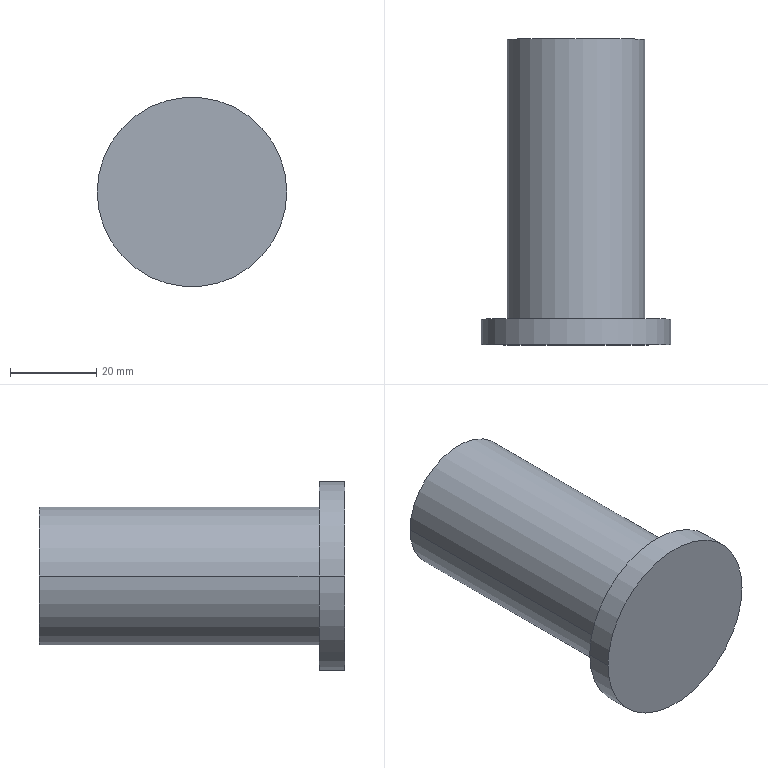Part | STEP file | Main ejector | 1 solid | 7 faces | box 44 x 71 x 44 mm | volume 61399 mm3 | cylinder 4 | plane 3 | commonest cylinder face diameters 32 x2 44 x2
STEP:
#1=CARTESIAN_POINT('',(0.,0.,0.));
#2=DIRECTION('',(0.,0.,1.));
#3=DIRECTION('',(1.,0.,0.));
#4=AXIS2_PLACEMENT_3D('',#1,#2,#3);
#5=CARTESIAN_POINT('',(-16.,6.,0.));
#6=VERTEX_POINT('',#5);
#7=CARTESIAN_POINT('',(16.,6.,0.));
#8=VERTEX_POINT('',#7);
#9=CARTESIAN_POINT('',(0.,6.,0.));
#10=DIRECTION('',(0.,1.,0.));
#11=DIRECTION('',(-1.,0.,0.));
#12=AXIS2_PLACEMENT_3D('',#9,#10,#11);
#13=CIRCLE('',#12,16.);
#14=CARTESIAN_POINT('',(0.,71.,0.));
#15=DIRECTION('',(0.,1.,0.));
#16=DIRECTION('',(-1.,0.,0.));
#17=AXIS2_PLACEMENT_3D('',#14,#15,#16);
#18=CYLINDRICAL_SURFACE('',#17,16.);
#19=CARTESIAN_POINT('',(0.,-65.));
#20=DIRECTION('',(1.,0.));
#21=VECTOR('',#20,1.);
#22=LINE('',#19,#21);
#23=(GEOMETRIC_REPRESENTATION_CONTEXT(2)PARAMETRIC_REPRESENTATION_CONTEXT()REPRESENTATION_CONTEXT('',''));
#24=DEFINITIONAL_REPRESENTATION('',(#22),#23);
#25=PCURVE('',#18,#24);
#26=CARTESIAN_POINT('',(-22.,6.,0.));
#27=DIRECTION('',(0.,1.,0.));
#28=DIRECTION('',(-1.,0.,0.));
#29=AXIS2_PLACEMENT_3D('',#26,#27,#28);
#30=PLANE('',#29);
#31=CARTESIAN_POINT('',(-22.,0.));
#32=DIRECTION('',(1.,0.));
#33=AXIS2_PLACEMENT_2D('',#31,#32);
#34=CIRCLE('',#33,16.);
#35=(GEOMETRIC_REPRESENTATION_CONTEXT(2)PARAMETRIC_REPRESENTATION_CONTEXT()REPRESENTATION_CONTEXT('',''));
#36=DEFINITIONAL_REPRESENTATION('',(#34),#35);
#37=PCURVE('',#30,#36);
#38=SURFACE_CURVE('',#13,(#25,#37),.PCURVE_S1.);
#39=EDGE_CURVE('',#6,#8,#38,.T.);
#40=ORIENTED_EDGE('',*,*,#39,.T.);
#41=CARTESIAN_POINT('',(16.,71.,0.));
#42=VERTEX_POINT('',#41);
#43=CARTESIAN_POINT('',(16.,71.,0.));
#44=DIRECTION('',(0.,1.,0.));
#45=VECTOR('',#44,1.);
#46=LINE('',#43,#45);
#47=CARTESIAN_POINT('',(3.142,0.));
#48=DIRECTION('',(0.,1.));
#49=VECTOR('',#48,1.);
#50=LINE('',#47,#49);
#51=(GEOMETRIC_REPRESENTATION_CONTEXT(2)PARAMETRIC_REPRESENTATION_CONTEXT()REPRESENTATION_CONTEXT('',''));
#52=DEFINITIONAL_REPRESENTATION('',(#50),#51);
#53=PCURVE('',#18,#52);
#54=CARTESIAN_POINT('',(0.,71.,0.));
#55=DIRECTION('',(0.,1.,0.));
#56=DIRECTION('',(-1.,0.,0.));
#57=AXIS2_PLACEMENT_3D('',#54,#55,#56);
#58=CYLINDRICAL_SURFACE('',#57,16.);
#59=CARTESIAN_POINT('',(3.142,0.));
#60=DIRECTION('',(0.,1.));
#61=VECTOR('',#60,1.);
#62=LINE('',#59,#61);
#63=(GEOMETRIC_REPRESENTATION_CONTEXT(2)PARAMETRIC_REPRESENTATION_CONTEXT()REPRESENTATION_CONTEXT('',''));
#64=DEFINITIONAL_REPRESENTATION('',(#62),#63);
#65=PCURVE('',#58,#64);
#66=SURFACE_CURVE('',#46,(#53,#65),.PCURVE_S1.);
#67=EDGE_CURVE('',#8,#42,#66,.T.);
#68=ORIENTED_EDGE('',*,*,#67,.T.);
#69=CARTESIAN_POINT('',(-16.,71.,0.));
#70=VERTEX_POINT('',#69);
#71=CARTESIAN_POINT('',(0.,71.,0.));
#72=DIRECTION('',(0.,1.,0.));
#73=DIRECTION('',(-1.,0.,0.));
#74=AXIS2_PLACEMENT_3D('',#71,#72,#73);
#75=CIRCLE('',#74,16.);
#76=CARTESIAN_POINT('',(0.,0.));
#77=DIRECTION('',(1.,0.));
#78=VECTOR('',#77,1.);
#79=LINE('',#76,#78);
#80=(GEOMETRIC_REPRESENTATION_CONTEXT(2)PARAMETRIC_REPRESENTATION_CONTEXT()REPRESENTATION_CONTEXT('',''));
#81=DEFINITIONAL_REPRESENTATION('',(#79),#80);
#82=PCURVE('',#18,#81);
#83=CARTESIAN_POINT('',(-16.,71.,0.));
#84=DIRECTION('',(0.,1.,0.));
#85=DIRECTION('',(-1.,0.,0.));
#86=AXIS2_PLACEMENT_3D('',#83,#84,#85);
#87=PLANE('',#86);
#88=CARTESIAN_POINT('',(-16.,0.));
#89=DIRECTION('',(1.,0.));
#90=AXIS2_PLACEMENT_2D('',#88,#89);
#91=CIRCLE('',#90,16.);
#92=(GEOMETRIC_REPRESENTATION_CONTEXT(2)PARAMETRIC_REPRESENTATION_CONTEXT()REPRESENTATION_CONTEXT('',''));
#93=DEFINITIONAL_REPRESENTATION('',(#91),#92);
#94=PCURVE('',#87,#93);
#95=SURFACE_CURVE('',#75,(#82,#94),.PCURVE_S1.);
#96=EDGE_CURVE('',#70,#42,#95,.T.);
#97=ORIENTED_EDGE('',*,*,#96,.F.);
#98=CARTESIAN_POINT('',(-16.,71.,0.));
#99=DIRECTION('',(0.,1.,0.));
#100=VECTOR('',#99,1.);
#101=LINE('',#98,#100);
#102=CARTESIAN_POINT('',(0.,0.));
#103=DIRECTION('',(0.,1.));
#104=VECTOR('',#103,1.);
#105=LINE('',#102,#104);
#106=(GEOMETRIC_REPRESENTATION_CONTEXT(2)PARAMETRIC_REPRESENTATION_CONTEXT()REPRESENTATION_CONTEXT('',''));
#107=DEFINITIONAL_REPRESENTATION('',(#105),#106);
#108=PCURVE('',#18,#107);
#109=CARTESIAN_POINT('',(6.283,0.));
#110=DIRECTION('',(0.,1.));
#111=VECTOR('',#110,1.);
#112=LINE('',#109,#111);
#113=(GEOMETRIC_REPRESENTATION_CONTEXT(2)PARAMETRIC_REPRESENTATION_CONTEXT()REPRESENTATION_CONTEXT('',''));
#114=DEFINITIONAL_REPRESENTATION('',(#112),#113);
#115=PCURVE('',#58,#114);
#116=SURFACE_CURVE('',#101,(#108,#115),.PCURVE_S1.);
#117=EDGE_CURVE('',#6,#70,#116,.T.);
#118=ORIENTED_EDGE('',*,*,#117,.F.);
#119=EDGE_LOOP('',(#40,#68,#97,#118));
#120=FACE_BOUND('',#119,.T.);
#121=ADVANCED_FACE('',(#120),#18,.T.);
#122=CARTESIAN_POINT('',(-22.,0.,0.));
#123=VERTEX_POINT('',#122);
#124=CARTESIAN_POINT('',(22.,0.,0.));
#125=VERTEX_POINT('',#124);
#126=CARTESIAN_POINT('',(0.,0.,0.));
#127=DIRECTION('',(0.,1.,0.));
#128=DIRECTION('',(-1.,0.,0.));
#129=AXIS2_PLACEMENT_3D('',#126,#127,#128);
#130=CIRCLE('',#129,22.);
#131=CARTESIAN_POINT('',(0.,71.,0.));
#132=DIRECTION('',(0.,1.,0.));
#133=DIRECTION('',(-1.,0.,0.));
#134=AXIS2_PLACEMENT_3D('',#131,#132,#133);
#135=CYLINDRICAL_SURFACE('',#134,22.);
#136=CARTESIAN_POINT('',(0.,-71.));
#137=DIRECTION('',(1.,0.));
#138=VECTOR('',#137,1.);
#139=LINE('',#136,#138);
#140=(GEOMETRIC_REPRESENTATION_CONTEXT(2)PARAMETRIC_REPRESENTATION_CONTEXT()REPRESENTATION_CONTEXT('',''));
#141=DEFINITIONAL_REPRESENTATION('',(#139),#140);
#142=PCURVE('',#135,#141);
#143=CARTESIAN_POINT('',(0.,0.,0.));
#144=DIRECTION('',(0.,-1.,0.));
#145=DIRECTION('',(1.,0.,0.));
#146=AXIS2_PLACEMENT_3D('',#143,#144,#145);
#147=PLANE('',#146);
#148=CARTESIAN_POINT('',(-22.,0.));
#149=CARTESIAN_POINT('',(-22.,38.105));
#150=CARTESIAN_POINT('',(11.,19.053));
#151=CARTESIAN_POINT('',(44.,0.));
#152=CARTESIAN_POINT('',(11.,-19.053));
#153=CARTESIAN_POINT('',(-22.,-38.105));
#154=CARTESIAN_POINT('',(-22.,0.));
#155=(BOUNDED_CURVE()B_SPLINE_CURVE(2,(#148,#149,#150,#151,#152,#153,#154),.UNSPECIFIED.,.T.,.F.)B_SPLINE_CURVE_WITH_KNOTS((1,2,2,2,2,1),(-2.094,0.,2.094,4.189,6.283,8.378),.UNSPECIFIED.)CURVE()GEOMETRIC_REPRESENTATION_ITEM()RATIONAL_B_SPLINE_CURVE((1.,0.5,1.,0.5,1.,0.5,1.))REPRESENTATION_ITEM(''));
#156=(GEOMETRIC_REPRESENTATION_CONTEXT(2)PARAMETRIC_REPRESENTATION_CONTEXT()REPRESENTATION_CONTEXT('',''));
#157=DEFINITIONAL_REPRESENTATION('',(#155),#156);
#158=PCURVE('',#147,#157);
#159=SURFACE_CURVE('',#130,(#142,#158),.PCURVE_S1.);
#160=EDGE_CURVE('',#123,#125,#159,.T.);
#161=ORIENTED_EDGE('',*,*,#160,.T.);
#162=CARTESIAN_POINT('',(22.,6.,0.));
#163=VERTEX_POINT('',#162);
#164=CARTESIAN_POINT('',(22.,71.,0.));
#165=DIRECTION('',(0.,1.,0.));
#166=VECTOR('',#165,1.);
#167=LINE('',#164,#166);
#168=CARTESIAN_POINT('',(3.142,0.));
#169=DIRECTION('',(0.,1.));
#170=VECTOR('',#169,1.);
#171=LINE('',#168,#170);
#172=(GEOMETRIC_REPRESENTATION_CONTEXT(2)PARAMETRIC_REPRESENTATION_CONTEXT()REPRESENTATION_CONTEXT('',''));
#173=DEFINITIONAL_REPRESENTATION('',(#171),#172);
#174=PCURVE('',#135,#173);
#175=CARTESIAN_POINT('',(0.,71.,0.));
#176=DIRECTION('',(0.,1.,0.));
#177=DIRECTION('',(-1.,0.,0.));
#178=AXIS2_PLACEMENT_3D('',#175,#176,#177);
#179=CYLINDRICAL_SURFACE('',#178,22.);
#180=CARTESIAN_POINT('',(3.142,0.));
#181=DIRECTION('',(0.,1.));
#182=VECTOR('',#181,1.);
#183=LINE('',#180,#182);
#184=(GEOMETRIC_REPRESENTATION_CONTEXT(2)PARAMETRIC_REPRESENTATION_CONTEXT()REPRESENTATION_CONTEXT('',''));
#185=DEFINITIONAL_REPRESENTATION('',(#183),#184);
#186=PCURVE('',#179,#185);
#187=SURFACE_CURVE('',#167,(#174,#186),.PCURVE_S1.);
#188=EDGE_CURVE('',#125,#163,#187,.T.);
#189=ORIENTED_EDGE('',*,*,#188,.T.);
#190=CARTESIAN_POINT('',(-22.,6.,0.));
#191=VERTEX_POINT('',#190);
#192=CARTESIAN_POINT('',(0.,6.,0.));
#193=DIRECTION('',(0.,1.,0.));
#194=DIRECTION('',(-1.,0.,0.));
#195=AXIS2_PLACEMENT_3D('',#192,#193,#194);
#196=CIRCLE('',#195,22.);
#197=CARTESIAN_POINT('',(0.,-65.));
#198=DIRECTION('',(1.,0.));
#199=VECTOR('',#198,1.);
#200=LINE('',#197,#199);
#201=(GEOMETRIC_REPRESENTATION_CONTEXT(2)PARAMETRIC_REPRESENTATION_CONTEXT()REPRESENTATION_CONTEXT('',''));
#202=DEFINITIONAL_REPRESENTATION('',(#200),#201);
#203=PCURVE('',#135,#202);
#204=CARTESIAN_POINT('',(-22.,0.));
#205=DIRECTION('',(1.,0.));
#206=AXIS2_PLACEMENT_2D('',#204,#205);
#207=CIRCLE('',#206,22.);
#208=(GEOMETRIC_REPRESENTATION_CONTEXT(2)PARAMETRIC_REPRESENTATION_CONTEXT()REPRESENTATION_CONTEXT('',''));
#209=DEFINITIONAL_REPRESENTATION('',(#207),#208);
#210=PCURVE('',#30,#209);
#211=SURFACE_CURVE('',#196,(#203,#210),.PCURVE_S1.);
#212=EDGE_CURVE('',#191,#163,#211,.T.);
#213=ORIENTED_EDGE('',*,*,#212,.F.);
#214=CARTESIAN_POINT('',(-22.,71.,0.));
#215=DIRECTION('',(0.,1.,0.));
#216=VECTOR('',#215,1.);
#217=LINE('',#214,#216);
#218=CARTESIAN_POINT('',(0.,0.));
#219=DIRECTION('',(0.,1.));
#220=VECTOR('',#219,1.);
#221=LINE('',#218,#220);
#222=(GEOMETRIC_REPRESENTATION_CONTEXT(2)PARAMETRIC_REPRESENTATION_CONTEXT()REPRESENTATION_CONTEXT('',''));
#223=DEFINITIONAL_REPRESENTATION('',(#221),#222);
#224=PCURVE('',#135,#223);
#225=CARTESIAN_POINT('',(6.283,0.));
#226=DIRECTION('',(0.,1.));
#227=VECTOR('',#226,1.);
#228=LINE('',#225,#227);
#229=(GEOMETRIC_REPRESENTATION_CONTEXT(2)PARAMETRIC_REPRESENTATION_CONTEXT()REPRESENTATION_CONTEXT('',''));
#230=DEFINITIONAL_REPRESENTATION('',(#228),#229);
#231=PCURVE('',#179,#230);
#232=SURFACE_CURVE('',#217,(#224,#231),.PCURVE_S1.);
#233=EDGE_CURVE('',#123,#191,#232,.T.);
#234=ORIENTED_EDGE('',*,*,#233,.F.);
#235=EDGE_LOOP('',(#161,#189,#213,#234));
#236=FACE_BOUND('',#235,.T.);
#237=ADVANCED_FACE('',(#236),#135,.T.);
#238=ORIENTED_EDGE('',*,*,#160,.F.);
#239=CARTESIAN_POINT('',(0.,0.,0.));
#240=DIRECTION('',(0.,1.,0.));
#241=DIRECTION('',(-1.,0.,0.));
#242=AXIS2_PLACEMENT_3D('',#239,#240,#241);
#243=CIRCLE('',#242,22.);
#244=CARTESIAN_POINT('',(-22.,0.));
#245=CARTESIAN_POINT('',(-22.,38.105));
#246=CARTESIAN_POINT('',(11.,19.053));
#247=CARTESIAN_POINT('',(44.,0.));
#248=CARTESIAN_POINT('',(11.,-19.053));
#249=CARTESIAN_POINT('',(-22.,-38.105));
#250=CARTESIAN_POINT('',(-22.,0.));
#251=(BOUNDED_CURVE()B_SPLINE_CURVE(2,(#244,#245,#246,#247,#248,#249,#250),.UNSPECIFIED.,.T.,.F.)B_SPLINE_CURVE_WITH_KNOTS((1,2,2,2,2,1),(-2.094,0.,2.094,4.189,6.283,8.378),.UNSPECIFIED.)CURVE()GEOMETRIC_REPRESENTATION_ITEM()RATIONAL_B_SPLINE_CURVE((1.,0.5,1.,0.5,1.,0.5,1.))REPRESENTATION_ITEM(''));
#252=(GEOMETRIC_REPRESENTATION_CONTEXT(2)PARAMETRIC_REPRESENTATION_CONTEXT()REPRESENTATION_CONTEXT('',''));
#253=DEFINITIONAL_REPRESENTATION('',(#251),#252);
#254=PCURVE('',#147,#253);
#255=CARTESIAN_POINT('',(0.,-71.));
#256=DIRECTION('',(1.,0.));
#257=VECTOR('',#256,1.);
#258=LINE('',#255,#257);
#259=(GEOMETRIC_REPRESENTATION_CONTEXT(2)PARAMETRIC_REPRESENTATION_CONTEXT()REPRESENTATION_CONTEXT('',''));
#260=DEFINITIONAL_REPRESENTATION('',(#258),#259);
#261=PCURVE('',#179,#260);
#262=SURFACE_CURVE('',#243,(#254,#261),.PCURVE_S1.);
#263=EDGE_CURVE('',#125,#123,#262,.T.);
#264=ORIENTED_EDGE('',*,*,#263,.F.);
#265=EDGE_LOOP('',(#238,#264));
#266=FACE_BOUND('',#265,.T.);
#267=ADVANCED_FACE('',(#266),#147,.T.);
#268=ORIENTED_EDGE('',*,*,#188,.F.);
#269=ORIENTED_EDGE('',*,*,#263,.T.);
#270=ORIENTED_EDGE('',*,*,#233,.T.);
#271=CARTESIAN_POINT('',(0.,6.,0.));
#272=DIRECTION('',(0.,1.,0.));
#273=DIRECTION('',(-1.,0.,0.));
#274=AXIS2_PLACEMENT_3D('',#271,#272,#273);
#275=CIRCLE('',#274,22.);
#276=CARTESIAN_POINT('',(0.,-65.));
#277=DIRECTION('',(1.,0.));
#278=VECTOR('',#277,1.);
#279=LINE('',#276,#278);
#280=(GEOMETRIC_REPRESENTATION_CONTEXT(2)PARAMETRIC_REPRESENTATION_CONTEXT()REPRESENTATION_CONTEXT('',''));
#281=DEFINITIONAL_REPRESENTATION('',(#279),#280);
#282=PCURVE('',#179,#281);
#283=CARTESIAN_POINT('',(-22.,0.));
#284=DIRECTION('',(1.,0.));
#285=AXIS2_PLACEMENT_2D('',#283,#284);
#286=CIRCLE('',#285,22.);
#287=(GEOMETRIC_REPRESENTATION_CONTEXT(2)PARAMETRIC_REPRESENTATION_CONTEXT()REPRESENTATION_CONTEXT('',''));
#288=DEFINITIONAL_REPRESENTATION('',(#286),#287);
#289=PCURVE('',#30,#288);
#290=SURFACE_CURVE('',#275,(#282,#289),.PCURVE_S1.);
#291=EDGE_CURVE('',#163,#191,#290,.T.);
#292=ORIENTED_EDGE('',*,*,#291,.F.);
#293=EDGE_LOOP('',(#268,#269,#270,#292));
#294=FACE_BOUND('',#293,.T.);
#295=ADVANCED_FACE('',(#294),#179,.T.);
#296=ORIENTED_EDGE('',*,*,#212,.T.);
#297=ORIENTED_EDGE('',*,*,#291,.T.);
#298=EDGE_LOOP('',(#296,#297));
#299=FACE_BOUND('',#298,.T.);
#300=ORIENTED_EDGE('',*,*,#39,.F.);
#301=CARTESIAN_POINT('',(0.,6.,0.));
#302=DIRECTION('',(0.,1.,0.));
#303=DIRECTION('',(-1.,0.,0.));
#304=AXIS2_PLACEMENT_3D('',#301,#302,#303);
#305=CIRCLE('',#304,16.);
#306=CARTESIAN_POINT('',(-22.,0.));
#307=DIRECTION('',(1.,0.));
#308=AXIS2_PLACEMENT_2D('',#306,#307);
#309=CIRCLE('',#308,16.);
#310=(GEOMETRIC_REPRESENTATION_CONTEXT(2)PARAMETRIC_REPRESENTATION_CONTEXT()REPRESENTATION_CONTEXT('',''));
#311=DEFINITIONAL_REPRESENTATION('',(#309),#310);
#312=PCURVE('',#30,#311);
#313=CARTESIAN_POINT('',(0.,-65.));
#314=DIRECTION('',(1.,0.));
#315=VECTOR('',#314,1.);
#316=LINE('',#313,#315);
#317=(GEOMETRIC_REPRESENTATION_CONTEXT(2)PARAMETRIC_REPRESENTATION_CONTEXT()REPRESENTATION_CONTEXT('',''));
#318=DEFINITIONAL_REPRESENTATION('',(#316),#317);
#319=PCURVE('',#58,#318);
#320=SURFACE_CURVE('',#305,(#312,#319),.PCURVE_S1.);
#321=EDGE_CURVE('',#8,#6,#320,.T.);
#322=ORIENTED_EDGE('',*,*,#321,.F.);
#323=EDGE_LOOP('',(#300,#322));
#324=FACE_BOUND('',#323,.T.);
#325=ADVANCED_FACE('',(#299,#324),#30,.T.);
#326=ORIENTED_EDGE('',*,*,#67,.F.);
#327=ORIENTED_EDGE('',*,*,#321,.T.);
#328=ORIENTED_EDGE('',*,*,#117,.T.);
#329=CARTESIAN_POINT('',(0.,71.,0.));
#330=DIRECTION('',(0.,1.,0.));
#331=DIRECTION('',(-1.,0.,0.));
#332=AXIS2_PLACEMENT_3D('',#329,#330,#331);
#333=CIRCLE('',#332,16.);
#334=CARTESIAN_POINT('',(0.,0.));
#335=DIRECTION('',(1.,0.));
#336=VECTOR('',#335,1.);
#337=LINE('',#334,#336);
#338=(GEOMETRIC_REPRESENTATION_CONTEXT(2)PARAMETRIC_REPRESENTATION_CONTEXT()REPRESENTATION_CONTEXT('',''));
#339=DEFINITIONAL_REPRESENTATION('',(#337),#338);
#340=PCURVE('',#58,#339);
#341=CARTESIAN_POINT('',(-16.,0.));
#342=DIRECTION('',(1.,0.));
#343=AXIS2_PLACEMENT_2D('',#341,#342);
#344=CIRCLE('',#343,16.);
#345=(GEOMETRIC_REPRESENTATION_CONTEXT(2)PARAMETRIC_REPRESENTATION_CONTEXT()REPRESENTATION_CONTEXT('',''));
#346=DEFINITIONAL_REPRESENTATION('',(#344),#345);
#347=PCURVE('',#87,#346);
#348=SURFACE_CURVE('',#333,(#340,#347),.PCURVE_S1.);
#349=EDGE_CURVE('',#42,#70,#348,.T.);
#350=ORIENTED_EDGE('',*,*,#349,.F.);
#351=EDGE_LOOP('',(#326,#327,#328,#350));
#352=FACE_BOUND('',#351,.T.);
#353=ADVANCED_FACE('',(#352),#58,.T.);
#354=ORIENTED_EDGE('',*,*,#96,.T.);
#355=ORIENTED_EDGE('',*,*,#349,.T.);
#356=EDGE_LOOP('',(#354,#355));
#357=FACE_BOUND('',#356,.T.);
#358=ADVANCED_FACE('',(#357),#87,.T.);
#359=CLOSED_SHELL('',(#121,#237,#267,#295,#325,#353,#358));
#360=MANIFOLD_SOLID_BREP('',#359);
#361=(LENGTH_UNIT()NAMED_UNIT(*)SI_UNIT(.MILLI.,.METRE.));
#362=UNCERTAINTY_MEASURE_WITH_UNIT(LENGTH_MEASURE(0.0000001),#361,'','');
#363=(NAMED_UNIT(*)PLANE_ANGLE_UNIT()SI_UNIT($,.RADIAN.));
#364=(NAMED_UNIT(*)SI_UNIT($,.STERADIAN.)SOLID_ANGLE_UNIT());
#365=(GEOMETRIC_REPRESENTATION_CONTEXT(3)GLOBAL_UNCERTAINTY_ASSIGNED_CONTEXT((#362))GLOBAL_UNIT_ASSIGNED_CONTEXT((#361,#363,#364))REPRESENTATION_CONTEXT('',''));
#366=ADVANCED_BREP_SHAPE_REPRESENTATION('',(#4,#360),#365);